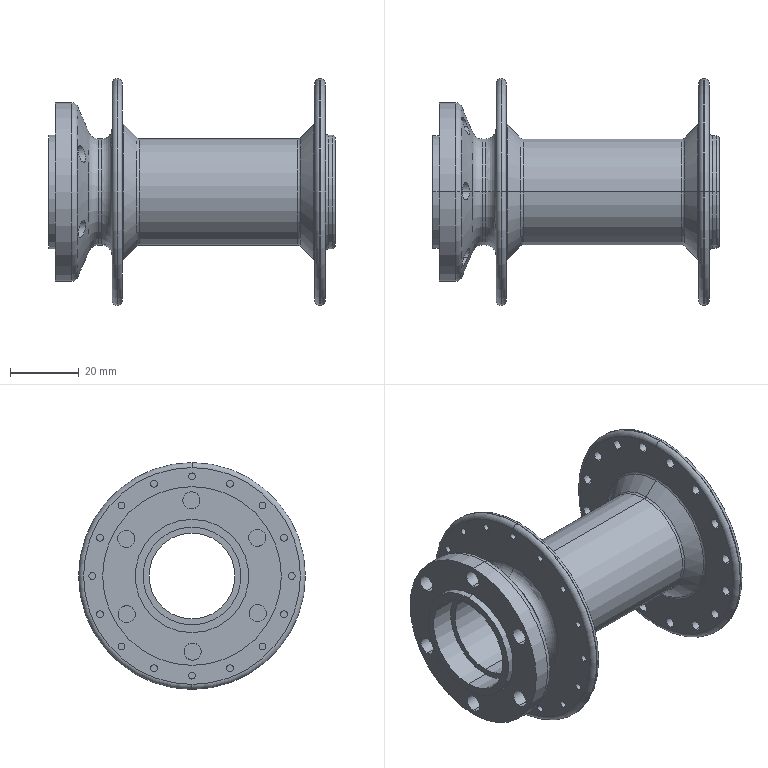Part | STEP file | KMX Front Hub | 1 solid | 137 faces | box 83.5 x 66 x 66 mm | volume 47544 mm3 | cylinder 96 | torus 26 | plane 9 | cone 6 | commonest cylinder face diameters 2 x32 3 x32 5 x12 28.5 x4 31 x4 33 x4